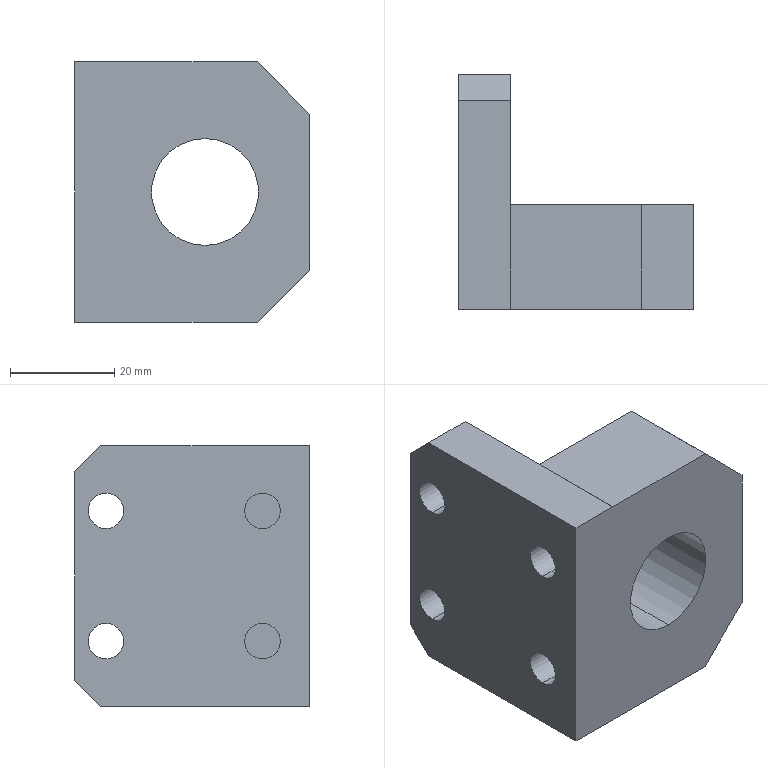Part | SolidWorks | features Chamfer 2, HoleWzd 2, Extrusion 1, ICE 1 | 1 solid | 25 faces | box 45 x 45 x 50 mm | volume 47153 mm3 | plane 15 | cylinder 10 | commonest cylinder face diameters 6.8 x8 20.5 x2
STEP:
#1=CARTESIAN_POINT('',(0.,16.5,15.9));
#2=VERTEX_POINT('',#1);
#3=CARTESIAN_POINT('',(0.,16.5,9.1));
#4=VERTEX_POINT('',#3);
#5=CARTESIAN_POINT('',(0.,16.5,12.5));
#6=DIRECTION('',(1.,0.,0.));
#7=DIRECTION('',(0.,0.,-1.));
#8=AXIS2_PLACEMENT_3D('',#5,#6,#7);
#9=CIRCLE('',#8,3.4);
#10=EDGE_CURVE('',#2,#4,#9,.T.);
#11=ORIENTED_EDGE('',*,*,#10,.F.);
#12=CARTESIAN_POINT('',(10.,16.5,15.9));
#13=VERTEX_POINT('',#12);
#14=CARTESIAN_POINT('',(10.,16.5,15.9));
#15=DIRECTION('',(1.,0.,0.));
#16=VECTOR('',#15,1000.);
#17=LINE('',#14,#16);
#18=EDGE_CURVE('',#2,#13,#17,.T.);
#19=ORIENTED_EDGE('',*,*,#18,.T.);
#20=CARTESIAN_POINT('',(10.,16.5,9.1));
#21=VERTEX_POINT('',#20);
#22=CARTESIAN_POINT('',(10.,16.5,12.5));
#23=DIRECTION('',(1.,0.,0.));
#24=DIRECTION('',(0.,0.,-1.));
#25=AXIS2_PLACEMENT_3D('',#22,#23,#24);
#26=CIRCLE('',#25,3.4);
#27=EDGE_CURVE('',#13,#21,#26,.T.);
#28=ORIENTED_EDGE('',*,*,#27,.T.);
#29=CARTESIAN_POINT('',(10.,16.5,9.1));
#30=DIRECTION('',(1.,0.,0.));
#31=VECTOR('',#30,1000.);
#32=LINE('',#29,#31);
#33=EDGE_CURVE('',#4,#21,#32,.T.);
#34=ORIENTED_EDGE('',*,*,#33,.F.);
#35=EDGE_LOOP('',(#11,#19,#28,#34));
#36=FACE_OUTER_BOUND('',#35,.T.);
#37=CARTESIAN_POINT('',(10.,16.5,12.5));
#38=DIRECTION('',(1.,0.,0.));
#39=DIRECTION('',(0.,0.,-1.));
#40=AXIS2_PLACEMENT_3D('',#37,#38,#39);
#41=CYLINDRICAL_SURFACE('',#40,3.4);
#42=ADVANCED_FACE('',(#36),#41,.F.);
#43=CARTESIAN_POINT('',(0.,16.5,-9.1));
#44=VERTEX_POINT('',#43);
#45=CARTESIAN_POINT('',(0.,16.5,-15.9));
#46=VERTEX_POINT('',#45);
#47=CARTESIAN_POINT('',(0.,16.5,-12.5));
#48=DIRECTION('',(1.,0.,0.));
#49=DIRECTION('',(0.,0.,-1.));
#50=AXIS2_PLACEMENT_3D('',#47,#48,#49);
#51=CIRCLE('',#50,3.4);
#52=EDGE_CURVE('',#44,#46,#51,.T.);
#53=ORIENTED_EDGE('',*,*,#52,.F.);
#54=CARTESIAN_POINT('',(10.,16.5,-9.1));
#55=VERTEX_POINT('',#54);
#56=CARTESIAN_POINT('',(10.,16.5,-9.1));
#57=DIRECTION('',(1.,0.,0.));
#58=VECTOR('',#57,1000.);
#59=LINE('',#56,#58);
#60=EDGE_CURVE('',#44,#55,#59,.T.);
#61=ORIENTED_EDGE('',*,*,#60,.T.);
#62=CARTESIAN_POINT('',(10.,16.5,-15.9));
#63=VERTEX_POINT('',#62);
#64=CARTESIAN_POINT('',(10.,16.5,-12.5));
#65=DIRECTION('',(1.,0.,0.));
#66=DIRECTION('',(0.,0.,-1.));
#67=AXIS2_PLACEMENT_3D('',#64,#65,#66);
#68=CIRCLE('',#67,3.4);
#69=EDGE_CURVE('',#55,#63,#68,.T.);
#70=ORIENTED_EDGE('',*,*,#69,.T.);
#71=CARTESIAN_POINT('',(10.,16.5,-15.9));
#72=DIRECTION('',(1.,0.,0.));
#73=VECTOR('',#72,1000.);
#74=LINE('',#71,#73);
#75=EDGE_CURVE('',#46,#63,#74,.T.);
#76=ORIENTED_EDGE('',*,*,#75,.F.);
#77=EDGE_LOOP('',(#53,#61,#70,#76));
#78=FACE_OUTER_BOUND('',#77,.T.);
#79=CARTESIAN_POINT('',(10.,16.5,-12.5));
#80=DIRECTION('',(1.,0.,0.));
#81=DIRECTION('',(0.,0.,-1.));
#82=AXIS2_PLACEMENT_3D('',#79,#80,#81);
#83=CYLINDRICAL_SURFACE('',#82,3.4);
#84=ADVANCED_FACE('',(#78),#83,.F.);
#85=CARTESIAN_POINT('',(0.,-13.5,15.9));
#86=VERTEX_POINT('',#85);
#87=CARTESIAN_POINT('',(0.,-13.5,9.1));
#88=VERTEX_POINT('',#87);
#89=CARTESIAN_POINT('',(0.,-13.5,12.5));
#90=DIRECTION('',(1.,0.,0.));
#91=DIRECTION('',(0.,0.,-1.));
#92=AXIS2_PLACEMENT_3D('',#89,#90,#91);
#93=CIRCLE('',#92,3.4);
#94=EDGE_CURVE('',#86,#88,#93,.T.);
#95=ORIENTED_EDGE('',*,*,#94,.F.);
#96=CARTESIAN_POINT('',(10.,-13.5,15.9));
#97=VERTEX_POINT('',#96);
#98=CARTESIAN_POINT('',(10.,-13.5,15.9));
#99=DIRECTION('',(1.,0.,0.));
#100=VECTOR('',#99,1000.);
#101=LINE('',#98,#100);
#102=EDGE_CURVE('',#86,#97,#101,.T.);
#103=ORIENTED_EDGE('',*,*,#102,.T.);
#104=CARTESIAN_POINT('',(10.,-13.5,9.1));
#105=VERTEX_POINT('',#104);
#106=CARTESIAN_POINT('',(10.,-13.5,12.5));
#107=DIRECTION('',(1.,0.,0.));
#108=DIRECTION('',(0.,0.,-1.));
#109=AXIS2_PLACEMENT_3D('',#106,#107,#108);
#110=CIRCLE('',#109,3.4);
#111=EDGE_CURVE('',#97,#105,#110,.T.);
#112=ORIENTED_EDGE('',*,*,#111,.T.);
#113=CARTESIAN_POINT('',(10.,-13.5,9.1));
#114=DIRECTION('',(1.,0.,0.));
#115=VECTOR('',#114,1000.);
#116=LINE('',#113,#115);
#117=EDGE_CURVE('',#88,#105,#116,.T.);
#118=ORIENTED_EDGE('',*,*,#117,.F.);
#119=EDGE_LOOP('',(#95,#103,#112,#118));
#120=FACE_OUTER_BOUND('',#119,.T.);
#121=CARTESIAN_POINT('',(10.,-13.5,12.5));
#122=DIRECTION('',(1.,0.,0.));
#123=DIRECTION('',(0.,0.,-1.));
#124=AXIS2_PLACEMENT_3D('',#121,#122,#123);
#125=CYLINDRICAL_SURFACE('',#124,3.4);
#126=ADVANCED_FACE('',(#120),#125,.F.);
#127=CARTESIAN_POINT('',(0.,-13.5,-9.1));
#128=VERTEX_POINT('',#127);
#129=CARTESIAN_POINT('',(0.,-13.5,-15.9));
#130=VERTEX_POINT('',#129);
#131=CARTESIAN_POINT('',(0.,-13.5,-12.5));
#132=DIRECTION('',(1.,0.,0.));
#133=DIRECTION('',(0.,0.,-1.));
#134=AXIS2_PLACEMENT_3D('',#131,#132,#133);
#135=CIRCLE('',#134,3.4);
#136=EDGE_CURVE('',#128,#130,#135,.T.);
#137=ORIENTED_EDGE('',*,*,#136,.F.);
#138=CARTESIAN_POINT('',(10.,-13.5,-9.1));
#139=VERTEX_POINT('',#138);
#140=CARTESIAN_POINT('',(10.,-13.5,-9.1));
#141=DIRECTION('',(1.,0.,0.));
#142=VECTOR('',#141,1000.);
#143=LINE('',#140,#142);
#144=EDGE_CURVE('',#128,#139,#143,.T.);
#145=ORIENTED_EDGE('',*,*,#144,.T.);
#146=CARTESIAN_POINT('',(10.,-13.5,-15.9));
#147=VERTEX_POINT('',#146);
#148=CARTESIAN_POINT('',(10.,-13.5,-12.5));
#149=DIRECTION('',(1.,0.,0.));
#150=DIRECTION('',(0.,0.,-1.));
#151=AXIS2_PLACEMENT_3D('',#148,#149,#150);
#152=CIRCLE('',#151,3.4);
#153=EDGE_CURVE('',#139,#147,#152,.T.);
#154=ORIENTED_EDGE('',*,*,#153,.T.);
#155=CARTESIAN_POINT('',(10.,-13.5,-15.9));
#156=DIRECTION('',(1.,0.,0.));
#157=VECTOR('',#156,1000.);
#158=LINE('',#155,#157);
#159=EDGE_CURVE('',#130,#147,#158,.T.);
#160=ORIENTED_EDGE('',*,*,#159,.F.);
#161=EDGE_LOOP('',(#137,#145,#154,#160));
#162=FACE_OUTER_BOUND('',#161,.T.);
#163=CARTESIAN_POINT('',(10.,-13.5,-12.5));
#164=DIRECTION('',(1.,0.,0.));
#165=DIRECTION('',(0.,0.,-1.));
#166=AXIS2_PLACEMENT_3D('',#163,#164,#165);
#167=CYLINDRICAL_SURFACE('',#166,3.4);
#168=ADVANCED_FACE('',(#162),#167,.F.);
#169=CARTESIAN_POINT('',(25.,-2.5,10.25));
#170=VERTEX_POINT('',#169);
#171=CARTESIAN_POINT('',(25.,-2.5,-10.25));
#172=VERTEX_POINT('',#171);
#173=CARTESIAN_POINT('',(25.,-2.5,0.));
#174=DIRECTION('',(0.,-1.,0.));
#175=DIRECTION('',(0.,0.,-1.));
#176=AXIS2_PLACEMENT_3D('',#173,#174,#175);
#177=CIRCLE('',#176,10.25);
#178=EDGE_CURVE('',#170,#172,#177,.T.);
#179=ORIENTED_EDGE('',*,*,#178,.F.);
#180=CARTESIAN_POINT('',(25.,-22.5,10.25));
#181=VERTEX_POINT('',#180);
#182=CARTESIAN_POINT('',(25.,-22.5,10.25));
#183=DIRECTION('',(0.,-1.,0.));
#184=VECTOR('',#183,1000.);
#185=LINE('',#182,#184);
#186=EDGE_CURVE('',#170,#181,#185,.T.);
#187=ORIENTED_EDGE('',*,*,#186,.T.);
#188=CARTESIAN_POINT('',(25.,-22.5,-10.25));
#189=VERTEX_POINT('',#188);
#190=CARTESIAN_POINT('',(25.,-22.5,0.));
#191=DIRECTION('',(0.,-1.,0.));
#192=DIRECTION('',(0.,0.,-1.));
#193=AXIS2_PLACEMENT_3D('',#190,#191,#192);
#194=CIRCLE('',#193,10.25);
#195=EDGE_CURVE('',#181,#189,#194,.T.);
#196=ORIENTED_EDGE('',*,*,#195,.T.);
#197=CARTESIAN_POINT('',(25.,-22.5,-10.25));
#198=DIRECTION('',(0.,-1.,0.));
#199=VECTOR('',#198,1000.);
#200=LINE('',#197,#199);
#201=EDGE_CURVE('',#172,#189,#200,.T.);
#202=ORIENTED_EDGE('',*,*,#201,.F.);
#203=EDGE_LOOP('',(#179,#187,#196,#202));
#204=FACE_OUTER_BOUND('',#203,.T.);
#205=CARTESIAN_POINT('',(25.,-22.5,0.));
#206=DIRECTION('',(0.,-1.,0.));
#207=DIRECTION('',(0.,0.,-1.));
#208=AXIS2_PLACEMENT_3D('',#205,#206,#207);
#209=CYLINDRICAL_SURFACE('',#208,10.25);
#210=ADVANCED_FACE('',(#204),#209,.F.);
#211=CARTESIAN_POINT('',(0.,-22.5,-25.));
#212=VERTEX_POINT('',#211);
#213=CARTESIAN_POINT('',(0.,17.5,-25.));
#214=VERTEX_POINT('',#213);
#215=CARTESIAN_POINT('',(0.,22.5,-25.));
#216=DIRECTION('',(0.,1.,0.));
#217=VECTOR('',#216,1000.);
#218=LINE('',#215,#217);
#219=EDGE_CURVE('',#212,#214,#218,.T.);
#220=ORIENTED_EDGE('',*,*,#219,.T.);
#221=CARTESIAN_POINT('',(10.,17.5,-25.));
#222=VERTEX_POINT('',#221);
#223=CARTESIAN_POINT('',(10.,17.5,-25.));
#224=DIRECTION('',(1.,0.,0.));
#225=VECTOR('',#224,1000.);
#226=LINE('',#223,#225);
#227=EDGE_CURVE('',#214,#222,#226,.T.);
#228=ORIENTED_EDGE('',*,*,#227,.T.);
#229=CARTESIAN_POINT('',(10.,-2.5,-25.));
#230=VERTEX_POINT('',#229);
#231=CARTESIAN_POINT('',(10.,22.5,-25.));
#232=DIRECTION('',(0.,1.,0.));
#233=VECTOR('',#232,1000.);
#234=LINE('',#231,#233);
#235=EDGE_CURVE('',#230,#222,#234,.T.);
#236=ORIENTED_EDGE('',*,*,#235,.F.);
#237=CARTESIAN_POINT('',(35.,-2.5,-25.));
#238=VERTEX_POINT('',#237);
#239=CARTESIAN_POINT('',(45.,-2.5,-25.));
#240=DIRECTION('',(-1.,0.,0.));
#241=VECTOR('',#240,1000.);
#242=LINE('',#239,#241);
#243=EDGE_CURVE('',#238,#230,#242,.T.);
#244=ORIENTED_EDGE('',*,*,#243,.F.);
#245=CARTESIAN_POINT('',(35.,-22.5,-25.));
#246=VERTEX_POINT('',#245);
#247=CARTESIAN_POINT('',(35.,-22.5,-25.));
#248=DIRECTION('',(0.,-1.,0.));
#249=VECTOR('',#248,1000.);
#250=LINE('',#247,#249);
#251=EDGE_CURVE('',#238,#246,#250,.T.);
#252=ORIENTED_EDGE('',*,*,#251,.T.);
#253=CARTESIAN_POINT('',(10.,-22.5,-25.));
#254=DIRECTION('',(-1.,0.,0.));
#255=VECTOR('',#254,1000.);
#256=LINE('',#253,#255);
#257=EDGE_CURVE('',#246,#212,#256,.T.);
#258=ORIENTED_EDGE('',*,*,#257,.T.);
#259=EDGE_LOOP('',(#220,#228,#236,#244,#252,#258));
#260=FACE_OUTER_BOUND('',#259,.T.);
#261=CARTESIAN_POINT('',(10.,22.5,-25.));
#262=DIRECTION('',(0.,0.,1.));
#263=DIRECTION('',(0.,-1.,0.));
#264=AXIS2_PLACEMENT_3D('',#261,#262,#263);
#265=PLANE('',#264);
#266=ADVANCED_FACE('',(#260),#265,.F.);
#267=CARTESIAN_POINT('',(10.,22.5,-20.));
#268=VERTEX_POINT('',#267);
#269=CARTESIAN_POINT('',(10.,22.5,20.));
#270=VERTEX_POINT('',#269);
#271=CARTESIAN_POINT('',(10.,22.5,25.));
#272=DIRECTION('',(0.,0.,1.));
#273=VECTOR('',#272,1000.);
#274=LINE('',#271,#273);
#275=EDGE_CURVE('',#268,#270,#274,.T.);
#276=ORIENTED_EDGE('',*,*,#275,.F.);
#277=CARTESIAN_POINT('',(0.,22.5,-20.));
#278=VERTEX_POINT('',#277);
#279=CARTESIAN_POINT('',(10.,22.5,-20.));
#280=DIRECTION('',(-1.,0.,0.));
#281=VECTOR('',#280,1000.);
#282=LINE('',#279,#281);
#283=EDGE_CURVE('',#268,#278,#282,.T.);
#284=ORIENTED_EDGE('',*,*,#283,.T.);
#285=CARTESIAN_POINT('',(0.,22.5,20.));
#286=VERTEX_POINT('',#285);
#287=CARTESIAN_POINT('',(0.,22.5,25.));
#288=DIRECTION('',(0.,0.,1.));
#289=VECTOR('',#288,1000.);
#290=LINE('',#287,#289);
#291=EDGE_CURVE('',#278,#286,#290,.T.);
#292=ORIENTED_EDGE('',*,*,#291,.T.);
#293=CARTESIAN_POINT('',(10.,22.5,20.));
#294=DIRECTION('',(1.,0.,0.));
#295=VECTOR('',#294,1000.);
#296=LINE('',#293,#295);
#297=EDGE_CURVE('',#286,#270,#296,.T.);
#298=ORIENTED_EDGE('',*,*,#297,.T.);
#299=EDGE_LOOP('',(#276,#284,#292,#298));
#300=FACE_OUTER_BOUND('',#299,.T.);
#301=CARTESIAN_POINT('',(10.,22.5,25.));
#302=DIRECTION('',(0.,-1.,0.));
#303=DIRECTION('',(0.,0.,-1.));
#304=AXIS2_PLACEMENT_3D('',#301,#302,#303);
#305=PLANE('',#304);
#306=ADVANCED_FACE('',(#300),#305,.F.);
#307=CARTESIAN_POINT('',(10.,17.5,25.));
#308=VERTEX_POINT('',#307);
#309=CARTESIAN_POINT('',(10.,-22.5,25.));
#310=VERTEX_POINT('',#309);
#311=CARTESIAN_POINT('',(10.,22.5,25.));
#312=DIRECTION('',(0.,-1.,0.));
#313=VECTOR('',#312,1000.);
#314=LINE('',#311,#313);
#315=EDGE_CURVE('',#308,#310,#314,.T.);
#316=ORIENTED_EDGE('',*,*,#315,.F.);
#317=CARTESIAN_POINT('',(0.,17.5,25.));
#318=VERTEX_POINT('',#317);
#319=CARTESIAN_POINT('',(10.,17.5,25.));
#320=DIRECTION('',(-1.,0.,0.));
#321=VECTOR('',#320,1000.);
#322=LINE('',#319,#321);
#323=EDGE_CURVE('',#308,#318,#322,.T.);
#324=ORIENTED_EDGE('',*,*,#323,.T.);
#325=CARTESIAN_POINT('',(0.,-22.5,25.));
#326=VERTEX_POINT('',#325);
#327=CARTESIAN_POINT('',(0.,22.5,25.));
#328=DIRECTION('',(0.,-1.,0.));
#329=VECTOR('',#328,1000.);
#330=LINE('',#327,#329);
#331=EDGE_CURVE('',#318,#326,#330,.T.);
#332=ORIENTED_EDGE('',*,*,#331,.T.);
#333=CARTESIAN_POINT('',(10.,-22.5,25.));
#334=DIRECTION('',(-1.,0.,0.));
#335=VECTOR('',#334,1000.);
#336=LINE('',#333,#335);
#337=EDGE_CURVE('',#310,#326,#336,.T.);
#338=ORIENTED_EDGE('',*,*,#337,.F.);
#339=EDGE_LOOP('',(#316,#324,#332,#338));
#340=FACE_OUTER_BOUND('',#339,.T.);
#341=CARTESIAN_POINT('',(10.,22.5,25.));
#342=DIRECTION('',(0.,0.,-1.));
#343=DIRECTION('',(0.,1.,0.));
#344=AXIS2_PLACEMENT_3D('',#341,#342,#343);
#345=PLANE('',#344);
#346=ADVANCED_FACE('',(#340),#345,.F.);
#347=CARTESIAN_POINT('',(25.,-22.5,0.));
#348=DIRECTION('',(0.,-1.,0.));
#349=DIRECTION('',(0.,0.,-1.));
#350=AXIS2_PLACEMENT_3D('',#347,#348,#349);
#351=CIRCLE('',#350,10.25);
#352=EDGE_CURVE('',#189,#181,#351,.T.);
#353=ORIENTED_EDGE('',*,*,#352,.F.);
#354=ORIENTED_EDGE('',*,*,#195,.F.);
#355=EDGE_LOOP('',(#353,#354));
#356=FACE_BOUND('',#355,.T.);
#357=ORIENTED_EDGE('',*,*,#257,.F.);
#358=CARTESIAN_POINT('',(45.,-22.5,-15.));
#359=VERTEX_POINT('',#358);
#360=CARTESIAN_POINT('',(45.,-22.5,-15.));
#361=DIRECTION('',(0.7071,0.,0.7071));
#362=VECTOR('',#361,1000.);
#363=LINE('',#360,#362);
#364=EDGE_CURVE('',#246,#359,#363,.T.);
#365=ORIENTED_EDGE('',*,*,#364,.T.);
#366=CARTESIAN_POINT('',(45.,-22.5,14.938));
#367=VERTEX_POINT('',#366);
#368=CARTESIAN_POINT('',(45.,-22.5,24.938));
#369=DIRECTION('',(0.,0.,-1.));
#370=VECTOR('',#369,1000.);
#371=LINE('',#368,#370);
#372=EDGE_CURVE('',#367,#359,#371,.T.);
#373=ORIENTED_EDGE('',*,*,#372,.F.);
#374=CARTESIAN_POINT('',(35.,-22.5,24.938));
#375=VERTEX_POINT('',#374);
#376=CARTESIAN_POINT('',(45.,-22.5,14.938));
#377=DIRECTION('',(-0.7071,0.,0.7071));
#378=VECTOR('',#377,1000.);
#379=LINE('',#376,#378);
#380=EDGE_CURVE('',#367,#375,#379,.T.);
#381=ORIENTED_EDGE('',*,*,#380,.T.);
#382=CARTESIAN_POINT('',(10.,-22.5,24.938));
#383=VERTEX_POINT('',#382);
#384=CARTESIAN_POINT('',(45.,-22.5,24.938));
#385=DIRECTION('',(-1.,0.,0.));
#386=VECTOR('',#385,1000.);
#387=LINE('',#384,#386);
#388=EDGE_CURVE('',#375,#383,#387,.T.);
#389=ORIENTED_EDGE('',*,*,#388,.T.);
#390=CARTESIAN_POINT('',(10.,-22.5,25.));
#391=DIRECTION('',(0.,0.,-1.));
#392=VECTOR('',#391,1000.);
#393=LINE('',#390,#392);
#394=EDGE_CURVE('',#310,#383,#393,.T.);
#395=ORIENTED_EDGE('',*,*,#394,.F.);
#396=ORIENTED_EDGE('',*,*,#337,.T.);
#397=CARTESIAN_POINT('',(0.,-22.5,25.));
#398=DIRECTION('',(0.,0.,-1.));
#399=VECTOR('',#398,1000.);
#400=LINE('',#397,#399);
#401=EDGE_CURVE('',#326,#212,#400,.T.);
#402=ORIENTED_EDGE('',*,*,#401,.T.);
#403=EDGE_LOOP('',(#357,#365,#373,#381,#389,#395,#396,#402));
#404=FACE_OUTER_BOUND('',#403,.T.);
#405=CARTESIAN_POINT('',(10.,-22.5,25.));
#406=DIRECTION('',(0.,1.,0.));
#407=DIRECTION('',(0.,0.,1.));
#408=AXIS2_PLACEMENT_3D('',#405,#406,#407);
#409=PLANE('',#408);
#410=ADVANCED_FACE('',(#356,#404),#409,.F.);
#411=CARTESIAN_POINT('',(10.,16.5,12.5));
#412=DIRECTION('',(1.,0.,0.));
#413=DIRECTION('',(0.,0.,-1.));
#414=AXIS2_PLACEMENT_3D('',#411,#412,#413);
#415=CIRCLE('',#414,3.4);
#416=EDGE_CURVE('',#21,#13,#415,.T.);
#417=ORIENTED_EDGE('',*,*,#416,.F.);
#418=ORIENTED_EDGE('',*,*,#27,.F.);
#419=EDGE_LOOP('',(#417,#418));
#420=FACE_BOUND('',#419,.T.);
#421=CARTESIAN_POINT('',(10.,16.5,-12.5));
#422=DIRECTION('',(1.,0.,0.));
#423=DIRECTION('',(0.,0.,-1.));
#424=AXIS2_PLACEMENT_3D('',#421,#422,#423);
#425=CIRCLE('',#424,3.4);
#426=EDGE_CURVE('',#63,#55,#425,.T.);
#427=ORIENTED_EDGE('',*,*,#426,.F.);
#428=ORIENTED_EDGE('',*,*,#69,.F.);
#429=EDGE_LOOP('',(#427,#428));
#430=FACE_BOUND('',#429,.T.);
#431=ORIENTED_EDGE('',*,*,#235,.T.);
#432=CARTESIAN_POINT('',(10.,21.25,-21.25));
#433=DIRECTION('',(0.,0.7071,0.7071));
#434=VECTOR('',#433,1000.);
#435=LINE('',#432,#434);
#436=EDGE_CURVE('',#222,#268,#435,.T.);
#437=ORIENTED_EDGE('',*,*,#436,.T.);
#438=ORIENTED_EDGE('',*,*,#275,.T.);
#439=CARTESIAN_POINT('',(10.,21.25,21.25));
#440=DIRECTION('',(0.,-0.7071,0.7071));
#441=VECTOR('',#440,1000.);
#442=LINE('',#439,#441);
#443=EDGE_CURVE('',#270,#308,#442,.T.);
#444=ORIENTED_EDGE('',*,*,#443,.T.);
#445=ORIENTED_EDGE('',*,*,#315,.T.);
#446=ORIENTED_EDGE('',*,*,#394,.T.);
#447=CARTESIAN_POINT('',(10.,-2.5,24.938));
#448=VERTEX_POINT('',#447);
#449=CARTESIAN_POINT('',(10.,-2.5,24.938));
#450=DIRECTION('',(0.,-1.,0.));
#451=VECTOR('',#450,1000.);
#452=LINE('',#449,#451);
#453=EDGE_CURVE('',#448,#383,#452,.T.);
#454=ORIENTED_EDGE('',*,*,#453,.F.);
#455=CARTESIAN_POINT('',(10.,-2.5,24.938));
#456=DIRECTION('',(0.,0.,1.));
#457=VECTOR('',#456,1000.);
#458=LINE('',#455,#457);
#459=EDGE_CURVE('',#230,#448,#458,.T.);
#460=ORIENTED_EDGE('',*,*,#459,.F.);
#461=EDGE_LOOP('',(#431,#437,#438,#444,#445,#446,#454,#460));
#462=FACE_OUTER_BOUND('',#461,.T.);
#463=CARTESIAN_POINT('',(10.,0.,0.));
#464=DIRECTION('',(1.,0.,0.));
#465=DIRECTION('',(0.,0.,-1.));
#466=AXIS2_PLACEMENT_3D('',#463,#464,#465);
#467=PLANE('',#466);
#468=ADVANCED_FACE('',(#420,#430,#462),#467,.T.);
#469=CARTESIAN_POINT('',(0.,16.5,12.5));
#470=DIRECTION('',(1.,0.,0.));
#471=DIRECTION('',(0.,0.,-1.));
#472=AXIS2_PLACEMENT_3D('',#469,#470,#471);
#473=CIRCLE('',#472,3.4);
#474=EDGE_CURVE('',#4,#2,#473,.T.);
#475=ORIENTED_EDGE('',*,*,#474,.T.);
#476=ORIENTED_EDGE('',*,*,#10,.T.);
#477=EDGE_LOOP('',(#475,#476));
#478=FACE_BOUND('',#477,.T.);
#479=CARTESIAN_POINT('',(0.,16.5,-12.5));
#480=DIRECTION('',(1.,0.,0.));
#481=DIRECTION('',(0.,0.,-1.));
#482=AXIS2_PLACEMENT_3D('',#479,#480,#481);
#483=CIRCLE('',#482,3.4);
#484=EDGE_CURVE('',#46,#44,#483,.T.);
#485=ORIENTED_EDGE('',*,*,#484,.T.);
#486=ORIENTED_EDGE('',*,*,#52,.T.);
#487=EDGE_LOOP('',(#485,#486));
#488=FACE_BOUND('',#487,.T.);
#489=CARTESIAN_POINT('',(0.,-13.5,12.5));
#490=DIRECTION('',(1.,0.,0.));
#491=DIRECTION('',(0.,0.,-1.));
#492=AXIS2_PLACEMENT_3D('',#489,#490,#491);
#493=CIRCLE('',#492,3.4);
#494=EDGE_CURVE('',#88,#86,#493,.T.);
#495=ORIENTED_EDGE('',*,*,#494,.T.);
#496=ORIENTED_EDGE('',*,*,#94,.T.);
#497=EDGE_LOOP('',(#495,#496));
#498=FACE_BOUND('',#497,.T.);
#499=CARTESIAN_POINT('',(0.,-13.5,-12.5));
#500=DIRECTION('',(1.,0.,0.));
#501=DIRECTION('',(0.,0.,-1.));
#502=AXIS2_PLACEMENT_3D('',#499,#500,#501);
#503=CIRCLE('',#502,3.4);
#504=EDGE_CURVE('',#130,#128,#503,.T.);
#505=ORIENTED_EDGE('',*,*,#504,.T.);
#506=ORIENTED_EDGE('',*,*,#136,.T.);
#507=EDGE_LOOP('',(#505,#506));
#508=FACE_BOUND('',#507,.T.);
#509=ORIENTED_EDGE('',*,*,#291,.F.);
#510=CARTESIAN_POINT('',(0.,22.5,-20.));
#511=DIRECTION('',(0.,-0.7071,-0.7071));
#512=VECTOR('',#511,1000.);
#513=LINE('',#510,#512);
#514=EDGE_CURVE('',#278,#214,#513,.T.);
#515=ORIENTED_EDGE('',*,*,#514,.T.);
#516=ORIENTED_EDGE('',*,*,#219,.F.);
#517=ORIENTED_EDGE('',*,*,#401,.F.);
#518=ORIENTED_EDGE('',*,*,#331,.F.);
#519=CARTESIAN_POINT('',(0.,17.5,25.));
#520=DIRECTION('',(0.,0.7071,-0.7071));
#521=VECTOR('',#520,1000.);
#522=LINE('',#519,#521);
#523=EDGE_CURVE('',#318,#286,#522,.T.);
#524=ORIENTED_EDGE('',*,*,#523,.T.);
#525=EDGE_LOOP('',(#509,#515,#516,#517,#518,#524));
#526=FACE_OUTER_BOUND('',#525,.T.);
#527=CARTESIAN_POINT('',(0.,0.,0.));
#528=DIRECTION('',(1.,0.,0.));
#529=DIRECTION('',(0.,0.,-1.));
#530=AXIS2_PLACEMENT_3D('',#527,#528,#529);
#531=PLANE('',#530);
#532=ADVANCED_FACE('',(#478,#488,#498,#508,#526),#531,.F.);
#533=CARTESIAN_POINT('',(25.,-2.5,0.));
#534=DIRECTION('',(0.,-1.,0.));
#535=DIRECTION('',(0.,0.,-1.));
#536=AXIS2_PLACEMENT_3D('',#533,#534,#535);
#537=CIRCLE('',#536,10.25);
#538=EDGE_CURVE('',#172,#170,#537,.T.);
#539=ORIENTED_EDGE('',*,*,#538,.T.);
#540=ORIENTED_EDGE('',*,*,#178,.T.);
#541=EDGE_LOOP('',(#539,#540));
#542=FACE_BOUND('',#541,.T.);
#543=CARTESIAN_POINT('',(45.,-2.5,-15.));
#544=VERTEX_POINT('',#543);
#545=CARTESIAN_POINT('',(45.,-2.5,14.938));
#546=VERTEX_POINT('',#545);
#547=CARTESIAN_POINT('',(45.,-2.5,24.938));
#548=DIRECTION('',(0.,0.,1.));
#549=VECTOR('',#548,1000.);
#550=LINE('',#547,#549);
#551=EDGE_CURVE('',#544,#546,#550,.T.);
#552=ORIENTED_EDGE('',*,*,#551,.F.);
#553=CARTESIAN_POINT('',(45.,-2.5,-15.));
#554=DIRECTION('',(-0.7071,0.,-0.7071));
#555=VECTOR('',#554,1000.);
#556=LINE('',#553,#555);
#557=EDGE_CURVE('',#544,#238,#556,.T.);
#558=ORIENTED_EDGE('',*,*,#557,.T.);
#559=ORIENTED_EDGE('',*,*,#243,.T.);
#560=ORIENTED_EDGE('',*,*,#459,.T.);
#561=CARTESIAN_POINT('',(35.,-2.5,24.938));
#562=VERTEX_POINT('',#561);
#563=CARTESIAN_POINT('',(45.,-2.5,24.938));
#564=DIRECTION('',(-1.,0.,0.));
#565=VECTOR('',#564,1000.);
#566=LINE('',#563,#565);
#567=EDGE_CURVE('',#562,#448,#566,.T.);
#568=ORIENTED_EDGE('',*,*,#567,.F.);
#569=CARTESIAN_POINT('',(45.,-2.5,14.938));
#570=DIRECTION('',(0.7071,0.,-0.7071));
#571=VECTOR('',#570,1000.);
#572=LINE('',#569,#571);
#573=EDGE_CURVE('',#562,#546,#572,.T.);
#574=ORIENTED_EDGE('',*,*,#573,.T.);
#575=EDGE_LOOP('',(#552,#558,#559,#560,#568,#574));
#576=FACE_OUTER_BOUND('',#575,.T.);
#577=CARTESIAN_POINT('',(45.,-2.5,24.938));
#578=DIRECTION('',(0.,-1.,0.));
#579=DIRECTION('',(0.,0.,-1.));
#580=AXIS2_PLACEMENT_3D('',#577,#578,#579);
#581=PLANE('',#580);
#582=ADVANCED_FACE('',(#542,#576),#581,.F.);
#583=ORIENTED_EDGE('',*,*,#388,.F.);
#584=CARTESIAN_POINT('',(35.,-2.5,24.938));
#585=DIRECTION('',(0.,1.,0.));
#586=VECTOR('',#585,1000.);
#587=LINE('',#584,#586);
#588=EDGE_CURVE('',#375,#562,#587,.T.);
#589=ORIENTED_EDGE('',*,*,#588,.T.);
#590=ORIENTED_EDGE('',*,*,#567,.T.);
#591=ORIENTED_EDGE('',*,*,#453,.T.);
#592=EDGE_LOOP('',(#583,#589,#590,#591));
#593=FACE_OUTER_BOUND('',#592,.T.);
#594=CARTESIAN_POINT('',(45.,-2.5,24.938));
#595=DIRECTION('',(0.,0.,-1.));
#596=DIRECTION('',(0.,1.,0.));
#597=AXIS2_PLACEMENT_3D('',#594,#595,#596);
#598=PLANE('',#597);
#599=ADVANCED_FACE('',(#593),#598,.F.);
#600=ORIENTED_EDGE('',*,*,#372,.T.);
#601=CARTESIAN_POINT('',(45.,-2.5,-15.));
#602=DIRECTION('',(0.,1.,0.));
#603=VECTOR('',#602,1000.);
#604=LINE('',#601,#603);
#605=EDGE_CURVE('',#359,#544,#604,.T.);
#606=ORIENTED_EDGE('',*,*,#605,.T.);
#607=ORIENTED_EDGE('',*,*,#551,.T.);
#608=CARTESIAN_POINT('',(45.,-22.5,14.938));
#609=DIRECTION('',(0.,-1.,0.));
#610=VECTOR('',#609,1000.);
#611=LINE('',#608,#610);
#612=EDGE_CURVE('',#546,#367,#611,.T.);
#613=ORIENTED_EDGE('',*,*,#612,.T.);
#614=EDGE_LOOP('',(#600,#606,#607,#613));
#615=FACE_OUTER_BOUND('',#614,.T.);
#616=CARTESIAN_POINT('',(45.,0.,0.));
#617=DIRECTION('',(1.,0.,0.));
#618=DIRECTION('',(0.,0.,-1.));
#619=AXIS2_PLACEMENT_3D('',#616,#617,#618);
#620=PLANE('',#619);
#621=ADVANCED_FACE('',(#615),#620,.T.);
#622=ORIENTED_EDGE('',*,*,#186,.F.);
#623=ORIENTED_EDGE('',*,*,#538,.F.);
#624=ORIENTED_EDGE('',*,*,#201,.T.);
#625=ORIENTED_EDGE('',*,*,#352,.T.);
#626=EDGE_LOOP('',(#622,#623,#624,#625));
#627=FACE_OUTER_BOUND('',#626,.T.);
#628=CARTESIAN_POINT('',(25.,-22.5,0.));
#629=DIRECTION('',(0.,-1.,0.));
#630=DIRECTION('',(0.,0.,-1.));
#631=AXIS2_PLACEMENT_3D('',#628,#629,#630);
#632=CYLINDRICAL_SURFACE('',#631,10.25);
#633=ADVANCED_FACE('',(#627),#632,.F.);
#634=CARTESIAN_POINT('',(10.,-13.5,-12.5));
#635=DIRECTION('',(1.,0.,0.));
#636=DIRECTION('',(0.,0.,-1.));
#637=AXIS2_PLACEMENT_3D('',#634,#635,#636);
#638=CIRCLE('',#637,3.4);
#639=EDGE_CURVE('',#147,#139,#638,.T.);
#640=ORIENTED_EDGE('',*,*,#639,.F.);
#641=ORIENTED_EDGE('',*,*,#153,.F.);
#642=EDGE_LOOP('',(#640,#641));
#643=FACE_OUTER_BOUND('',#642,.T.);
#644=CARTESIAN_POINT('',(10.,-10.1,-12.5));
#645=DIRECTION('',(1.,0.,0.));
#646=DIRECTION('',(0.,0.,-1.));
#647=AXIS2_PLACEMENT_3D('',#644,#645,#646);
#648=PLANE('',#647);
#649=ADVANCED_FACE('',(#643),#648,.F.);
#650=ORIENTED_EDGE('',*,*,#144,.F.);
#651=ORIENTED_EDGE('',*,*,#504,.F.);
#652=ORIENTED_EDGE('',*,*,#159,.T.);
#653=ORIENTED_EDGE('',*,*,#639,.T.);
#654=EDGE_LOOP('',(#650,#651,#652,#653));
#655=FACE_OUTER_BOUND('',#654,.T.);
#656=CARTESIAN_POINT('',(10.,-13.5,-12.5));
#657=DIRECTION('',(1.,0.,0.));
#658=DIRECTION('',(0.,0.,-1.));
#659=AXIS2_PLACEMENT_3D('',#656,#657,#658);
#660=CYLINDRICAL_SURFACE('',#659,3.4);
#661=ADVANCED_FACE('',(#655),#660,.F.);
#662=CARTESIAN_POINT('',(10.,-13.5,12.5));
#663=DIRECTION('',(1.,0.,0.));
#664=DIRECTION('',(0.,0.,-1.));
#665=AXIS2_PLACEMENT_3D('',#662,#663,#664);
#666=CIRCLE('',#665,3.4);
#667=EDGE_CURVE('',#105,#97,#666,.T.);
#668=ORIENTED_EDGE('',*,*,#667,.F.);
#669=ORIENTED_EDGE('',*,*,#111,.F.);
#670=EDGE_LOOP('',(#668,#669));
#671=FACE_OUTER_BOUND('',#670,.T.);
#672=CARTESIAN_POINT('',(10.,-10.1,12.5));
#673=DIRECTION('',(1.,0.,0.));
#674=DIRECTION('',(0.,0.,-1.));
#675=AXIS2_PLACEMENT_3D('',#672,#673,#674);
#676=PLANE('',#675);
#677=ADVANCED_FACE('',(#671),#676,.F.);
#678=ORIENTED_EDGE('',*,*,#102,.F.);
#679=ORIENTED_EDGE('',*,*,#494,.F.);
#680=ORIENTED_EDGE('',*,*,#117,.T.);
#681=ORIENTED_EDGE('',*,*,#667,.T.);
#682=EDGE_LOOP('',(#678,#679,#680,#681));
#683=FACE_OUTER_BOUND('',#682,.T.);
#684=CARTESIAN_POINT('',(10.,-13.5,12.5));
#685=DIRECTION('',(1.,0.,0.));
#686=DIRECTION('',(0.,0.,-1.));
#687=AXIS2_PLACEMENT_3D('',#684,#685,#686);
#688=CYLINDRICAL_SURFACE('',#687,3.4);
#689=ADVANCED_FACE('',(#683),#688,.F.);
#690=ORIENTED_EDGE('',*,*,#60,.F.);
#691=ORIENTED_EDGE('',*,*,#484,.F.);
#692=ORIENTED_EDGE('',*,*,#75,.T.);
#693=ORIENTED_EDGE('',*,*,#426,.T.);
#694=EDGE_LOOP('',(#690,#691,#692,#693));
#695=FACE_OUTER_BOUND('',#694,.T.);
#696=CARTESIAN_POINT('',(10.,16.5,-12.5));
#697=DIRECTION('',(1.,0.,0.));
#698=DIRECTION('',(0.,0.,-1.));
#699=AXIS2_PLACEMENT_3D('',#696,#697,#698);
#700=CYLINDRICAL_SURFACE('',#699,3.4);
#701=ADVANCED_FACE('',(#695),#700,.F.);
#702=ORIENTED_EDGE('',*,*,#18,.F.);
#703=ORIENTED_EDGE('',*,*,#474,.F.);
#704=ORIENTED_EDGE('',*,*,#33,.T.);
#705=ORIENTED_EDGE('',*,*,#416,.T.);
#706=EDGE_LOOP('',(#702,#703,#704,#705));
#707=FACE_OUTER_BOUND('',#706,.T.);
#708=CARTESIAN_POINT('',(10.,16.5,12.5));
#709=DIRECTION('',(1.,0.,0.));
#710=DIRECTION('',(0.,0.,-1.));
#711=AXIS2_PLACEMENT_3D('',#708,#709,#710);
#712=CYLINDRICAL_SURFACE('',#711,3.4);
#713=ADVANCED_FACE('',(#707),#712,.F.);
#714=ORIENTED_EDGE('',*,*,#364,.F.);
#715=ORIENTED_EDGE('',*,*,#251,.F.);
#716=ORIENTED_EDGE('',*,*,#557,.F.);
#717=ORIENTED_EDGE('',*,*,#605,.F.);
#718=EDGE_LOOP('',(#714,#715,#716,#717));
#719=FACE_OUTER_BOUND('',#718,.T.);
#720=CARTESIAN_POINT('',(45.,0.,-15.));
#721=DIRECTION('',(0.7071,0.,-0.7071));
#722=DIRECTION('',(0.,-1.,0.));
#723=AXIS2_PLACEMENT_3D('',#720,#721,#722);
#724=PLANE('',#723);
#725=ADVANCED_FACE('',(#719),#724,.T.);
#726=ORIENTED_EDGE('',*,*,#573,.F.);
#727=ORIENTED_EDGE('',*,*,#588,.F.);
#728=ORIENTED_EDGE('',*,*,#380,.F.);
#729=ORIENTED_EDGE('',*,*,#612,.F.);
#730=EDGE_LOOP('',(#726,#727,#728,#729));
#731=FACE_OUTER_BOUND('',#730,.T.);
#732=CARTESIAN_POINT('',(45.,0.,14.938));
#733=DIRECTION('',(0.7071,0.,0.7071));
#734=DIRECTION('',(0.,1.,0.));
#735=AXIS2_PLACEMENT_3D('',#732,#733,#734);
#736=PLANE('',#735);
#737=ADVANCED_FACE('',(#731),#736,.T.);
#738=ORIENTED_EDGE('',*,*,#436,.F.);
#739=ORIENTED_EDGE('',*,*,#227,.F.);
#740=ORIENTED_EDGE('',*,*,#514,.F.);
#741=ORIENTED_EDGE('',*,*,#283,.F.);
#742=EDGE_LOOP('',(#738,#739,#740,#741));
#743=FACE_OUTER_BOUND('',#742,.T.);
#744=CARTESIAN_POINT('',(10.,22.5,-20.));
#745=DIRECTION('',(0.,-0.7071,0.7071));
#746=DIRECTION('',(-1.,0.,0.));
#747=AXIS2_PLACEMENT_3D('',#744,#745,#746);
#748=PLANE('',#747);
#749=ADVANCED_FACE('',(#743),#748,.F.);
#750=ORIENTED_EDGE('',*,*,#443,.F.);
#751=ORIENTED_EDGE('',*,*,#297,.F.);
#752=ORIENTED_EDGE('',*,*,#523,.F.);
#753=ORIENTED_EDGE('',*,*,#323,.F.);
#754=EDGE_LOOP('',(#750,#751,#752,#753));
#755=FACE_OUTER_BOUND('',#754,.T.);
#756=CARTESIAN_POINT('',(10.,17.5,25.));
#757=DIRECTION('',(0.,-0.7071,-0.7071));
#758=DIRECTION('',(-1.,0.,0.));
#759=AXIS2_PLACEMENT_3D('',#756,#757,#758);
#760=PLANE('',#759);
#761=ADVANCED_FACE('',(#755),#760,.F.);
#762=CLOSED_SHELL('',(#42,#84,#126,#168,#210,#266,#306,#346,#410,#468,#532,#582,#599,#621,#633,#649,#661,#677,#689,#701,#713,#725,#737,#749,#761));
#763=MANIFOLD_SOLID_BREP('',#762);
#764=CARTESIAN_POINT('',(0.,0.,0.));
#765=DIRECTION('',(0.,0.,1.));
#766=DIRECTION('',(1.,0.,0.));
#767=AXIS2_PLACEMENT_3D('',#764,#765,#766);
#768=(LENGTH_UNIT()NAMED_UNIT(*)SI_UNIT(.MILLI.,.METRE.));
#769=UNCERTAINTY_MEASURE_WITH_UNIT(LENGTH_MEASURE(0.00001),#768,'','');
#770=(NAMED_UNIT(*)PLANE_ANGLE_UNIT()SI_UNIT($,.RADIAN.));
#771=(NAMED_UNIT(*)SI_UNIT($,.STERADIAN.)SOLID_ANGLE_UNIT());
#772=(GEOMETRIC_REPRESENTATION_CONTEXT(3)GLOBAL_UNCERTAINTY_ASSIGNED_CONTEXT((#769))GLOBAL_UNIT_ASSIGNED_CONTEXT((#768,#770,#771))REPRESENTATION_CONTEXT('',''));
#773=ADVANCED_BREP_SHAPE_REPRESENTATION('',(#763,#767),#772);